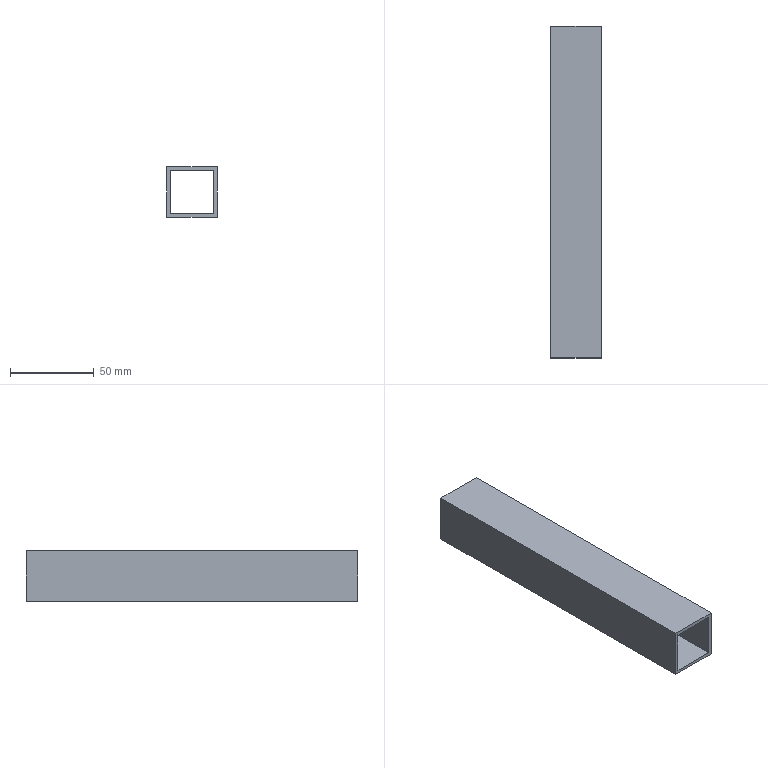Part | NX | features solid 2 | 1 solid | 10 faces | box 30 x 198.521 x 30 mm | volume 44469 mm3 | plane 10
STEP:
#1=CARTESIAN_POINT('',(245.839,716.479,-180.));
#2=VERTEX_POINT('',#1);
#3=CARTESIAN_POINT('',(245.839,915.,-180.));
#4=VERTEX_POINT('',#3);
#5=CARTESIAN_POINT('',(245.839,776.479,-180.));
#6=DIRECTION('',(0.,1.,0.));
#7=VECTOR('',#6,1000.);
#8=LINE('',#5,#7);
#9=EDGE_CURVE('',#2,#4,#8,.T.);
#10=ORIENTED_EDGE('',*,*,#9,.F.);
#11=CARTESIAN_POINT('',(275.839,716.479,-180.));
#12=VERTEX_POINT('',#11);
#13=CARTESIAN_POINT('',(275.839,716.479,-180.));
#14=DIRECTION('',(1.,0.,0.));
#15=VECTOR('',#14,1000.);
#16=LINE('',#13,#15);
#17=EDGE_CURVE('',#12,#2,#16,.F.);
#18=ORIENTED_EDGE('',*,*,#17,.F.);
#19=CARTESIAN_POINT('',(275.839,915.,-180.));
#20=VERTEX_POINT('',#19);
#21=CARTESIAN_POINT('',(275.839,776.479,-180.));
#22=DIRECTION('',(0.,-1.,0.));
#23=VECTOR('',#22,1000.);
#24=LINE('',#21,#23);
#25=EDGE_CURVE('',#12,#20,#24,.F.);
#26=ORIENTED_EDGE('',*,*,#25,.T.);
#27=CARTESIAN_POINT('',(275.839,915.,-180.));
#28=DIRECTION('',(1.,0.,0.));
#29=VECTOR('',#28,1000.);
#30=LINE('',#27,#29);
#31=EDGE_CURVE('',#20,#4,#30,.F.);
#32=ORIENTED_EDGE('',*,*,#31,.T.);
#33=EDGE_LOOP('',(#10,#18,#26,#32));
#34=FACE_BOUND('',#33,.T.);
#35=CARTESIAN_POINT('',(275.839,776.479,-180.));
#36=DIRECTION('',(0.,0.,1.));
#37=DIRECTION('',(0.,-1.,0.));
#38=AXIS2_PLACEMENT_3D('',#35,#36,#37);
#39=PLANE('',#38);
#40=ADVANCED_FACE('',(#34),#39,.T.);
#41=CARTESIAN_POINT('',(275.839,716.479,-210.));
#42=VERTEX_POINT('',#41);
#43=CARTESIAN_POINT('',(275.839,915.,-210.));
#44=VERTEX_POINT('',#43);
#45=CARTESIAN_POINT('',(275.839,776.479,-210.));
#46=DIRECTION('',(0.,1.,0.));
#47=VECTOR('',#46,1000.);
#48=LINE('',#45,#47);
#49=EDGE_CURVE('',#42,#44,#48,.T.);
#50=ORIENTED_EDGE('',*,*,#49,.F.);
#51=CARTESIAN_POINT('',(245.839,716.479,-210.));
#52=VERTEX_POINT('',#51);
#53=CARTESIAN_POINT('',(275.839,716.479,-210.));
#54=DIRECTION('',(1.,0.,0.));
#55=VECTOR('',#54,1000.);
#56=LINE('',#53,#55);
#57=EDGE_CURVE('',#42,#52,#56,.F.);
#58=ORIENTED_EDGE('',*,*,#57,.T.);
#59=CARTESIAN_POINT('',(245.839,915.,-210.));
#60=VERTEX_POINT('',#59);
#61=CARTESIAN_POINT('',(245.839,776.479,-210.));
#62=DIRECTION('',(0.,1.,0.));
#63=VECTOR('',#62,1000.);
#64=LINE('',#61,#63);
#65=EDGE_CURVE('',#52,#60,#64,.T.);
#66=ORIENTED_EDGE('',*,*,#65,.T.);
#67=CARTESIAN_POINT('',(395.,915.,-210.));
#68=DIRECTION('',(-1.,0.,0.));
#69=VECTOR('',#68,1000.);
#70=LINE('',#67,#69);
#71=EDGE_CURVE('',#60,#44,#70,.F.);
#72=ORIENTED_EDGE('',*,*,#71,.T.);
#73=EDGE_LOOP('',(#50,#58,#66,#72));
#74=FACE_BOUND('',#73,.T.);
#75=CARTESIAN_POINT('',(275.839,776.479,-210.));
#76=DIRECTION('',(0.,0.,1.));
#77=DIRECTION('',(0.,-1.,0.));
#78=AXIS2_PLACEMENT_3D('',#75,#76,#77);
#79=PLANE('',#78);
#80=ADVANCED_FACE('',(#74),#79,.F.);
#81=ORIENTED_EDGE('',*,*,#65,.F.);
#82=CARTESIAN_POINT('',(245.839,716.479,-210.));
#83=DIRECTION('',(0.,0.,-1.));
#84=VECTOR('',#83,1000.);
#85=LINE('',#82,#84);
#86=EDGE_CURVE('',#52,#2,#85,.F.);
#87=ORIENTED_EDGE('',*,*,#86,.T.);
#88=ORIENTED_EDGE('',*,*,#9,.T.);
#89=CARTESIAN_POINT('',(245.839,915.,-235.));
#90=DIRECTION('',(0.,0.,1.));
#91=VECTOR('',#90,1000.);
#92=LINE('',#89,#91);
#93=EDGE_CURVE('',#4,#60,#92,.F.);
#94=ORIENTED_EDGE('',*,*,#93,.T.);
#95=EDGE_LOOP('',(#81,#87,#88,#94));
#96=FACE_BOUND('',#95,.T.);
#97=CARTESIAN_POINT('',(245.839,776.479,-210.));
#98=DIRECTION('',(1.,0.,0.));
#99=DIRECTION('',(0.,1.,0.));
#100=AXIS2_PLACEMENT_3D('',#97,#98,#99);
#101=PLANE('',#100);
#102=ADVANCED_FACE('',(#96),#101,.F.);
#103=ORIENTED_EDGE('',*,*,#25,.F.);
#104=CARTESIAN_POINT('',(275.839,716.479,-210.));
#105=DIRECTION('',(0.,0.,-1.));
#106=VECTOR('',#105,1000.);
#107=LINE('',#104,#106);
#108=EDGE_CURVE('',#12,#42,#107,.T.);
#109=ORIENTED_EDGE('',*,*,#108,.T.);
#110=ORIENTED_EDGE('',*,*,#49,.T.);
#111=CARTESIAN_POINT('',(275.839,915.,-235.));
#112=DIRECTION('',(0.,0.,1.));
#113=VECTOR('',#112,1000.);
#114=LINE('',#111,#113);
#115=EDGE_CURVE('',#44,#20,#114,.T.);
#116=ORIENTED_EDGE('',*,*,#115,.T.);
#117=EDGE_LOOP('',(#103,#109,#110,#116));
#118=FACE_BOUND('',#117,.T.);
#119=CARTESIAN_POINT('',(275.839,776.479,-210.));
#120=DIRECTION('',(1.,0.,0.));
#121=DIRECTION('',(0.,1.,0.));
#122=AXIS2_PLACEMENT_3D('',#119,#120,#121);
#123=PLANE('',#122);
#124=ADVANCED_FACE('',(#118),#123,.T.);
#125=ORIENTED_EDGE('',*,*,#71,.F.);
#126=ORIENTED_EDGE('',*,*,#93,.F.);
#127=ORIENTED_EDGE('',*,*,#31,.F.);
#128=ORIENTED_EDGE('',*,*,#115,.F.);
#129=EDGE_LOOP('',(#125,#126,#127,#128));
#130=FACE_BOUND('',#129,.T.);
#131=CARTESIAN_POINT('',(247.839,915.,-182.));
#132=VERTEX_POINT('',#131);
#133=CARTESIAN_POINT('',(247.839,915.,-208.));
#134=VERTEX_POINT('',#133);
#135=CARTESIAN_POINT('',(247.839,915.,-235.));
#136=DIRECTION('',(0.,0.,1.));
#137=VECTOR('',#136,1000.);
#138=LINE('',#135,#137);
#139=EDGE_CURVE('',#132,#134,#138,.F.);
#140=ORIENTED_EDGE('',*,*,#139,.T.);
#141=CARTESIAN_POINT('',(273.839,915.,-208.));
#142=VERTEX_POINT('',#141);
#143=CARTESIAN_POINT('',(395.,915.,-208.));
#144=DIRECTION('',(-1.,0.,0.));
#145=VECTOR('',#144,1000.);
#146=LINE('',#143,#145);
#147=EDGE_CURVE('',#134,#142,#146,.F.);
#148=ORIENTED_EDGE('',*,*,#147,.T.);
#149=CARTESIAN_POINT('',(273.839,915.,-182.));
#150=VERTEX_POINT('',#149);
#151=CARTESIAN_POINT('',(273.839,915.,-235.));
#152=DIRECTION('',(0.,0.,1.));
#153=VECTOR('',#152,1000.);
#154=LINE('',#151,#153);
#155=EDGE_CURVE('',#142,#150,#154,.T.);
#156=ORIENTED_EDGE('',*,*,#155,.T.);
#157=CARTESIAN_POINT('',(275.839,915.,-182.));
#158=DIRECTION('',(1.,0.,0.));
#159=VECTOR('',#158,1000.);
#160=LINE('',#157,#159);
#161=EDGE_CURVE('',#150,#132,#160,.F.);
#162=ORIENTED_EDGE('',*,*,#161,.T.);
#163=EDGE_LOOP('',(#140,#148,#156,#162));
#164=FACE_BOUND('',#163,.T.);
#165=CARTESIAN_POINT('',(395.,915.,-235.));
#166=DIRECTION('',(0.,-1.,0.));
#167=DIRECTION('',(1.,0.,0.));
#168=AXIS2_PLACEMENT_3D('',#165,#166,#167);
#169=PLANE('',#168);
#170=ADVANCED_FACE('',(#130,#164),#169,.F.);
#171=CARTESIAN_POINT('',(273.839,716.479,-182.));
#172=VERTEX_POINT('',#171);
#173=CARTESIAN_POINT('',(273.839,776.479,-182.));
#174=DIRECTION('',(0.,-1.,0.));
#175=VECTOR('',#174,1000.);
#176=LINE('',#173,#175);
#177=EDGE_CURVE('',#172,#150,#176,.F.);
#178=ORIENTED_EDGE('',*,*,#177,.F.);
#179=CARTESIAN_POINT('',(247.839,716.479,-182.));
#180=VERTEX_POINT('',#179);
#181=CARTESIAN_POINT('',(275.839,716.479,-182.));
#182=DIRECTION('',(1.,0.,0.));
#183=VECTOR('',#182,1000.);
#184=LINE('',#181,#183);
#185=EDGE_CURVE('',#172,#180,#184,.F.);
#186=ORIENTED_EDGE('',*,*,#185,.T.);
#187=CARTESIAN_POINT('',(247.839,776.479,-182.));
#188=DIRECTION('',(0.,1.,0.));
#189=VECTOR('',#188,1000.);
#190=LINE('',#187,#189);
#191=EDGE_CURVE('',#180,#132,#190,.T.);
#192=ORIENTED_EDGE('',*,*,#191,.T.);
#193=ORIENTED_EDGE('',*,*,#161,.F.);
#194=EDGE_LOOP('',(#178,#186,#192,#193));
#195=FACE_BOUND('',#194,.T.);
#196=CARTESIAN_POINT('',(275.839,776.479,-182.));
#197=DIRECTION('',(0.,0.,1.));
#198=DIRECTION('',(0.,-1.,0.));
#199=AXIS2_PLACEMENT_3D('',#196,#197,#198);
#200=PLANE('',#199);
#201=ADVANCED_FACE('',(#195),#200,.F.);
#202=CARTESIAN_POINT('',(247.839,716.479,-208.));
#203=VERTEX_POINT('',#202);
#204=CARTESIAN_POINT('',(247.839,776.479,-208.));
#205=DIRECTION('',(0.,1.,0.));
#206=VECTOR('',#205,1000.);
#207=LINE('',#204,#206);
#208=EDGE_CURVE('',#203,#134,#207,.T.);
#209=ORIENTED_EDGE('',*,*,#208,.F.);
#210=CARTESIAN_POINT('',(273.839,716.479,-208.));
#211=VERTEX_POINT('',#210);
#212=CARTESIAN_POINT('',(275.839,716.479,-208.));
#213=DIRECTION('',(1.,0.,0.));
#214=VECTOR('',#213,1000.);
#215=LINE('',#212,#214);
#216=EDGE_CURVE('',#211,#203,#215,.F.);
#217=ORIENTED_EDGE('',*,*,#216,.F.);
#218=CARTESIAN_POINT('',(273.839,776.479,-208.));
#219=DIRECTION('',(0.,-1.,0.));
#220=VECTOR('',#219,1000.);
#221=LINE('',#218,#220);
#222=EDGE_CURVE('',#211,#142,#221,.F.);
#223=ORIENTED_EDGE('',*,*,#222,.T.);
#224=ORIENTED_EDGE('',*,*,#147,.F.);
#225=EDGE_LOOP('',(#209,#217,#223,#224));
#226=FACE_BOUND('',#225,.T.);
#227=CARTESIAN_POINT('',(275.839,776.479,-208.));
#228=DIRECTION('',(0.,0.,1.));
#229=DIRECTION('',(0.,-1.,0.));
#230=AXIS2_PLACEMENT_3D('',#227,#228,#229);
#231=PLANE('',#230);
#232=ADVANCED_FACE('',(#226),#231,.T.);
#233=ORIENTED_EDGE('',*,*,#191,.F.);
#234=CARTESIAN_POINT('',(247.839,716.479,-210.));
#235=DIRECTION('',(0.,0.,-1.));
#236=VECTOR('',#235,1000.);
#237=LINE('',#234,#236);
#238=EDGE_CURVE('',#203,#180,#237,.F.);
#239=ORIENTED_EDGE('',*,*,#238,.F.);
#240=ORIENTED_EDGE('',*,*,#208,.T.);
#241=ORIENTED_EDGE('',*,*,#139,.F.);
#242=EDGE_LOOP('',(#233,#239,#240,#241));
#243=FACE_BOUND('',#242,.T.);
#244=CARTESIAN_POINT('',(247.839,776.479,-210.));
#245=DIRECTION('',(1.,0.,0.));
#246=DIRECTION('',(0.,1.,0.));
#247=AXIS2_PLACEMENT_3D('',#244,#245,#246);
#248=PLANE('',#247);
#249=ADVANCED_FACE('',(#243),#248,.T.);
#250=ORIENTED_EDGE('',*,*,#222,.F.);
#251=CARTESIAN_POINT('',(273.839,716.479,-210.));
#252=DIRECTION('',(0.,0.,-1.));
#253=VECTOR('',#252,1000.);
#254=LINE('',#251,#253);
#255=EDGE_CURVE('',#172,#211,#254,.T.);
#256=ORIENTED_EDGE('',*,*,#255,.F.);
#257=ORIENTED_EDGE('',*,*,#177,.T.);
#258=ORIENTED_EDGE('',*,*,#155,.F.);
#259=EDGE_LOOP('',(#250,#256,#257,#258));
#260=FACE_BOUND('',#259,.T.);
#261=CARTESIAN_POINT('',(273.839,776.479,-210.));
#262=DIRECTION('',(1.,0.,0.));
#263=DIRECTION('',(0.,1.,0.));
#264=AXIS2_PLACEMENT_3D('',#261,#262,#263);
#265=PLANE('',#264);
#266=ADVANCED_FACE('',(#260),#265,.F.);
#267=ORIENTED_EDGE('',*,*,#17,.T.);
#268=ORIENTED_EDGE('',*,*,#86,.F.);
#269=ORIENTED_EDGE('',*,*,#57,.F.);
#270=ORIENTED_EDGE('',*,*,#108,.F.);
#271=EDGE_LOOP('',(#267,#268,#269,#270));
#272=FACE_BOUND('',#271,.T.);
#273=ORIENTED_EDGE('',*,*,#255,.T.);
#274=ORIENTED_EDGE('',*,*,#216,.T.);
#275=ORIENTED_EDGE('',*,*,#238,.T.);
#276=ORIENTED_EDGE('',*,*,#185,.F.);
#277=EDGE_LOOP('',(#273,#274,#275,#276));
#278=FACE_BOUND('',#277,.T.);
#279=CARTESIAN_POINT('',(275.839,716.479,-55.));
#280=DIRECTION('',(0.,-1.,0.));
#281=DIRECTION('',(1.,0.,0.));
#282=AXIS2_PLACEMENT_3D('',#279,#280,#281);
#283=PLANE('',#282);
#284=ADVANCED_FACE('',(#272,#278),#283,.T.);
#285=CLOSED_SHELL('',(#40,#80,#102,#124,#170,#201,#232,#249,#266,#284));
#286=MANIFOLD_SOLID_BREP('',#285);
#287=(LENGTH_UNIT()NAMED_UNIT(*)SI_UNIT(.MILLI.,.METRE.));
#288=UNCERTAINTY_MEASURE_WITH_UNIT(LENGTH_MEASURE(0.00001),#287,'','');
#289=(NAMED_UNIT(*)PLANE_ANGLE_UNIT()SI_UNIT($,.RADIAN.));
#290=(NAMED_UNIT(*)SI_UNIT($,.STERADIAN.)SOLID_ANGLE_UNIT());
#291=(GEOMETRIC_REPRESENTATION_CONTEXT(3)GLOBAL_UNCERTAINTY_ASSIGNED_CONTEXT((#288))GLOBAL_UNIT_ASSIGNED_CONTEXT((#287,#289,#290))REPRESENTATION_CONTEXT('',''));
#292=ADVANCED_BREP_SHAPE_REPRESENTATION('',(#286),#291);